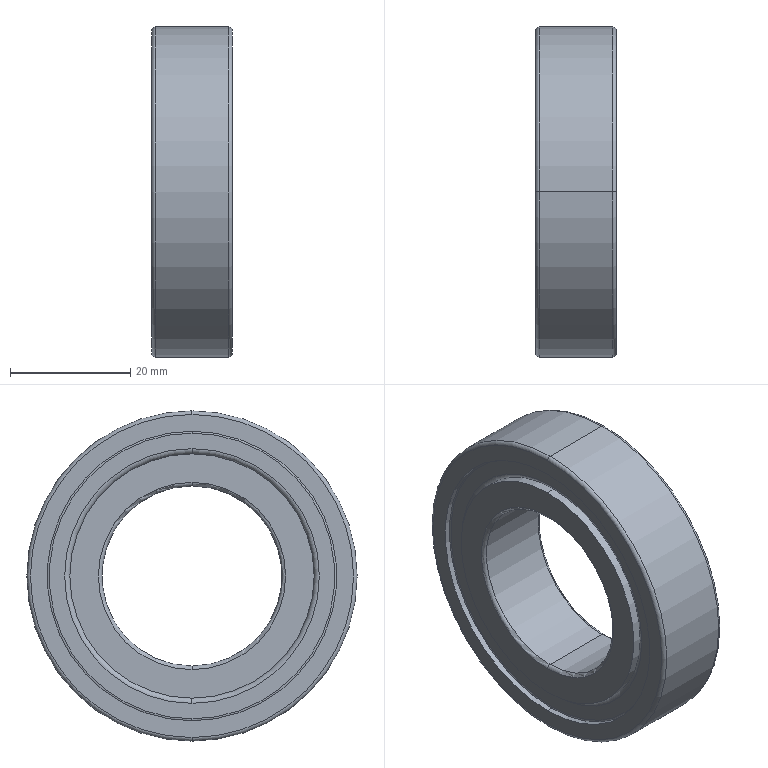Part | STEP file | Completa.sldasm-Part-110_Valor predeterminado | 1 solid | 42 faces | box 13.436 x 55 x 55 mm | volume 21253 mm3 | torus 16 | cylinder 16 | plane 10 | commonest cylinder face diameters 40.7 x4 48.225 x4 49.3 x4 30 x2 55 x2